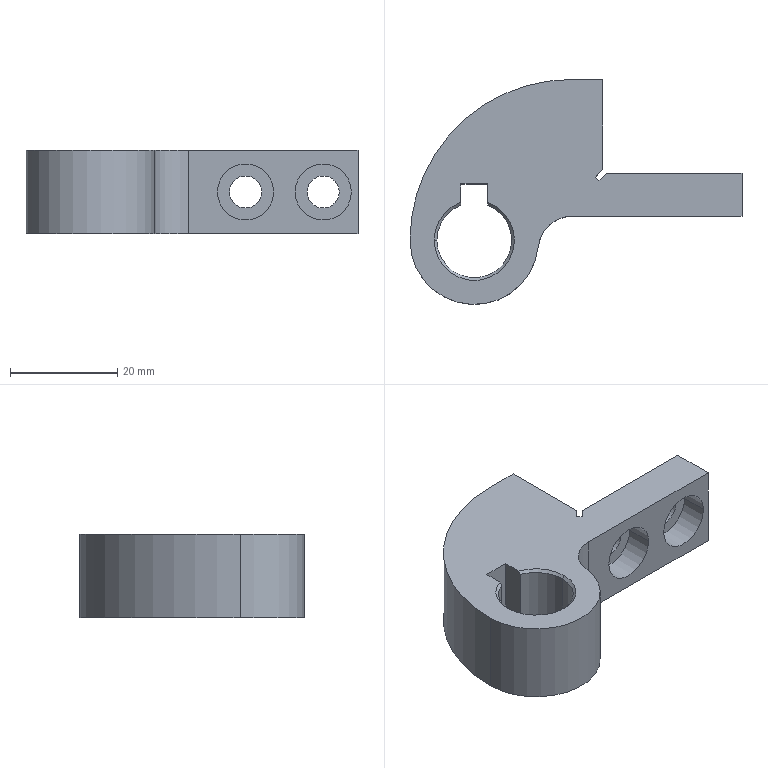Part | SolidWorks | features ICE 3, Chamfer 1, Extrusion 1 | 1 solid | 35 faces | box 62 x 42 x 15.5 mm | volume 16029 mm3 | plane 15 | cylinder 14 | cone 6 | commonest cylinder face diameters 6 x4 10.5 x4 14 x3 13 x1 24 x1 60 x1
STEP:
#1=CARTESIAN_POINT('',(-7.,0.,7.25));
#2=VERTEX_POINT('',#1);
#3=CARTESIAN_POINT('',(7.,0.,7.25));
#4=VERTEX_POINT('',#3);
#5=CARTESIAN_POINT('',(0.,0.,7.25));
#6=DIRECTION('',(0.,0.,1.));
#7=DIRECTION('',(1.,0.,0.));
#8=AXIS2_PLACEMENT_3D('',#5,#6,#7);
#9=CIRCLE('',#8,7.);
#10=EDGE_CURVE('',#2,#4,#9,.T.);
#11=ORIENTED_EDGE('',*,*,#10,.F.);
#12=CARTESIAN_POINT('',(-7.5,0.,7.75));
#13=VERTEX_POINT('',#12);
#14=CARTESIAN_POINT('',(-7.,0.,7.25));
#15=DIRECTION('',(-0.7071,0.,0.7071));
#16=VECTOR('',#15,1000.);
#17=LINE('',#14,#16);
#18=EDGE_CURVE('',#2,#13,#17,.T.);
#19=ORIENTED_EDGE('',*,*,#18,.T.);
#20=CARTESIAN_POINT('',(7.5,0.,7.75));
#21=VERTEX_POINT('',#20);
#22=CARTESIAN_POINT('',(0.,0.,7.75));
#23=DIRECTION('',(0.,0.,-1.));
#24=DIRECTION('',(1.,0.,0.));
#25=AXIS2_PLACEMENT_3D('',#22,#23,#24);
#26=CIRCLE('',#25,7.5);
#27=EDGE_CURVE('',#21,#13,#26,.T.);
#28=ORIENTED_EDGE('',*,*,#27,.F.);
#29=CARTESIAN_POINT('',(7.,0.,7.25));
#30=DIRECTION('',(0.7071,0.,0.7071));
#31=VECTOR('',#30,1000.);
#32=LINE('',#29,#31);
#33=EDGE_CURVE('',#4,#21,#32,.T.);
#34=ORIENTED_EDGE('',*,*,#33,.F.);
#35=EDGE_LOOP('',(#11,#19,#28,#34));
#36=FACE_OUTER_BOUND('',#35,.T.);
#37=CARTESIAN_POINT('',(0.,0.,7.25));
#38=DIRECTION('',(0.,0.,1.));
#39=DIRECTION('',(1.,0.,0.));
#40=AXIS2_PLACEMENT_3D('',#37,#38,#39);
#41=CONICAL_SURFACE('',#40,7.,0.7854);
#42=ADVANCED_FACE('',(#36),#41,.F.);
#43=CARTESIAN_POINT('',(2.5,6.538,7.25));
#44=VERTEX_POINT('',#43);
#45=CARTESIAN_POINT('',(0.,0.,7.25));
#46=DIRECTION('',(0.,0.,1.));
#47=DIRECTION('',(1.,0.,0.));
#48=AXIS2_PLACEMENT_3D('',#45,#46,#47);
#49=CIRCLE('',#48,7.);
#50=EDGE_CURVE('',#4,#44,#49,.T.);
#51=ORIENTED_EDGE('',*,*,#50,.F.);
#52=ORIENTED_EDGE('',*,*,#33,.T.);
#53=CARTESIAN_POINT('',(2.5,7.071,7.75));
#54=VERTEX_POINT('',#53);
#55=CARTESIAN_POINT('',(0.,0.,7.75));
#56=DIRECTION('',(0.,0.,-1.));
#57=DIRECTION('',(1.,0.,0.));
#58=AXIS2_PLACEMENT_3D('',#55,#56,#57);
#59=CIRCLE('',#58,7.5);
#60=EDGE_CURVE('',#54,#21,#59,.T.);
#61=ORIENTED_EDGE('',*,*,#60,.F.);
#62=CARTESIAN_POINT('',(2.5,6.538,7.25));
#63=CARTESIAN_POINT('',(2.5,6.716,7.416));
#64=CARTESIAN_POINT('',(2.5,6.894,7.583));
#65=CARTESIAN_POINT('',(2.5,7.071,7.75));
#66=B_SPLINE_CURVE_WITH_KNOTS('',3,(#62,#63,#64,#65),.UNSPECIFIED.,.F.,.F.,(4,4),(0.,0.0007306),.UNSPECIFIED.);
#67=EDGE_CURVE('',#44,#54,#66,.T.);
#68=ORIENTED_EDGE('',*,*,#67,.F.);
#69=EDGE_LOOP('',(#51,#52,#61,#68));
#70=FACE_OUTER_BOUND('',#69,.T.);
#71=CARTESIAN_POINT('',(0.,0.,7.25));
#72=DIRECTION('',(0.,0.,1.));
#73=DIRECTION('',(1.,0.,0.));
#74=AXIS2_PLACEMENT_3D('',#71,#72,#73);
#75=CONICAL_SURFACE('',#74,7.,0.7854);
#76=ADVANCED_FACE('',(#70),#75,.F.);
#77=CARTESIAN_POINT('',(7.,0.,-7.25));
#78=VERTEX_POINT('',#77);
#79=CARTESIAN_POINT('',(-7.,0.,-7.25));
#80=VERTEX_POINT('',#79);
#81=CARTESIAN_POINT('',(0.,0.,-7.25));
#82=DIRECTION('',(0.,0.,-1.));
#83=DIRECTION('',(1.,0.,0.));
#84=AXIS2_PLACEMENT_3D('',#81,#82,#83);
#85=CIRCLE('',#84,7.);
#86=EDGE_CURVE('',#78,#80,#85,.T.);
#87=ORIENTED_EDGE('',*,*,#86,.F.);
#88=CARTESIAN_POINT('',(7.5,0.,-7.75));
#89=VERTEX_POINT('',#88);
#90=CARTESIAN_POINT('',(7.5,0.,-7.75));
#91=DIRECTION('',(0.7071,0.,-0.7071));
#92=VECTOR('',#91,1000.);
#93=LINE('',#90,#92);
#94=EDGE_CURVE('',#78,#89,#93,.T.);
#95=ORIENTED_EDGE('',*,*,#94,.T.);
#96=CARTESIAN_POINT('',(-7.5,0.,-7.75));
#97=VERTEX_POINT('',#96);
#98=CARTESIAN_POINT('',(0.,0.,-7.75));
#99=DIRECTION('',(0.,0.,1.));
#100=DIRECTION('',(1.,0.,0.));
#101=AXIS2_PLACEMENT_3D('',#98,#99,#100);
#102=CIRCLE('',#101,7.5);
#103=EDGE_CURVE('',#97,#89,#102,.T.);
#104=ORIENTED_EDGE('',*,*,#103,.F.);
#105=CARTESIAN_POINT('',(-7.5,0.,-7.75));
#106=DIRECTION('',(-0.7071,0.,-0.7071));
#107=VECTOR('',#106,1000.);
#108=LINE('',#105,#107);
#109=EDGE_CURVE('',#80,#97,#108,.T.);
#110=ORIENTED_EDGE('',*,*,#109,.F.);
#111=EDGE_LOOP('',(#87,#95,#104,#110));
#112=FACE_OUTER_BOUND('',#111,.T.);
#113=CARTESIAN_POINT('',(0.,0.,-7.75));
#114=DIRECTION('',(0.,0.,-1.));
#115=DIRECTION('',(-1.,0.,0.));
#116=AXIS2_PLACEMENT_3D('',#113,#114,#115);
#117=CONICAL_SURFACE('',#116,7.5,0.7854);
#118=ADVANCED_FACE('',(#112),#117,.F.);
#119=CARTESIAN_POINT('',(-2.5,6.538,-7.25));
#120=VERTEX_POINT('',#119);
#121=CARTESIAN_POINT('',(0.,0.,-7.25));
#122=DIRECTION('',(0.,0.,-1.));
#123=DIRECTION('',(1.,0.,0.));
#124=AXIS2_PLACEMENT_3D('',#121,#122,#123);
#125=CIRCLE('',#124,7.);
#126=EDGE_CURVE('',#80,#120,#125,.T.);
#127=ORIENTED_EDGE('',*,*,#126,.F.);
#128=ORIENTED_EDGE('',*,*,#109,.T.);
#129=CARTESIAN_POINT('',(-2.5,7.071,-7.75));
#130=VERTEX_POINT('',#129);
#131=CARTESIAN_POINT('',(0.,0.,-7.75));
#132=DIRECTION('',(0.,0.,1.));
#133=DIRECTION('',(1.,0.,0.));
#134=AXIS2_PLACEMENT_3D('',#131,#132,#133);
#135=CIRCLE('',#134,7.5);
#136=EDGE_CURVE('',#130,#97,#135,.T.);
#137=ORIENTED_EDGE('',*,*,#136,.F.);
#138=CARTESIAN_POINT('',(-2.5,6.538,-7.25));
#139=CARTESIAN_POINT('',(-2.5,6.716,-7.416));
#140=CARTESIAN_POINT('',(-2.5,6.894,-7.583));
#141=CARTESIAN_POINT('',(-2.5,7.071,-7.75));
#142=B_SPLINE_CURVE_WITH_KNOTS('',3,(#138,#139,#140,#141),.UNSPECIFIED.,.F.,.F.,(4,4),(0.,0.0007306),.UNSPECIFIED.);
#143=EDGE_CURVE('',#120,#130,#142,.T.);
#144=ORIENTED_EDGE('',*,*,#143,.F.);
#145=EDGE_LOOP('',(#127,#128,#137,#144));
#146=FACE_OUTER_BOUND('',#145,.T.);
#147=CARTESIAN_POINT('',(0.,0.,-7.75));
#148=DIRECTION('',(0.,0.,-1.));
#149=DIRECTION('',(-1.,0.,0.));
#150=AXIS2_PLACEMENT_3D('',#147,#148,#149);
#151=CONICAL_SURFACE('',#150,7.5,0.7854);
#152=ADVANCED_FACE('',(#146),#151,.F.);
#153=CARTESIAN_POINT('',(38.25,9.5,0.));
#154=VERTEX_POINT('',#153);
#155=CARTESIAN_POINT('',(48.75,9.5,0.));
#156=VERTEX_POINT('',#155);
#157=CARTESIAN_POINT('',(43.5,9.5,0.));
#158=DIRECTION('',(0.,-1.,0.));
#159=DIRECTION('',(1.,0.,0.));
#160=AXIS2_PLACEMENT_3D('',#157,#158,#159);
#161=CIRCLE('',#160,5.25);
#162=EDGE_CURVE('',#154,#156,#161,.T.);
#163=ORIENTED_EDGE('',*,*,#162,.F.);
#164=CARTESIAN_POINT('',(38.25,4.5,0.));
#165=VERTEX_POINT('',#164);
#166=CARTESIAN_POINT('',(38.25,9.5,0.));
#167=DIRECTION('',(0.,-1.,0.));
#168=VECTOR('',#167,1000.);
#169=LINE('',#166,#168);
#170=EDGE_CURVE('',#154,#165,#169,.T.);
#171=ORIENTED_EDGE('',*,*,#170,.T.);
#172=CARTESIAN_POINT('',(48.75,4.5,0.));
#173=VERTEX_POINT('',#172);
#174=CARTESIAN_POINT('',(43.5,4.5,0.));
#175=DIRECTION('',(0.,-1.,0.));
#176=DIRECTION('',(1.,0.,0.));
#177=AXIS2_PLACEMENT_3D('',#174,#175,#176);
#178=CIRCLE('',#177,5.25);
#179=EDGE_CURVE('',#165,#173,#178,.T.);
#180=ORIENTED_EDGE('',*,*,#179,.T.);
#181=CARTESIAN_POINT('',(48.75,9.5,0.));
#182=DIRECTION('',(0.,-1.,0.));
#183=VECTOR('',#182,1000.);
#184=LINE('',#181,#183);
#185=EDGE_CURVE('',#156,#173,#184,.T.);
#186=ORIENTED_EDGE('',*,*,#185,.F.);
#187=EDGE_LOOP('',(#163,#171,#180,#186));
#188=FACE_OUTER_BOUND('',#187,.T.);
#189=CARTESIAN_POINT('',(43.5,9.5,0.));
#190=DIRECTION('',(0.,-1.,0.));
#191=DIRECTION('',(1.,0.,0.));
#192=AXIS2_PLACEMENT_3D('',#189,#190,#191);
#193=CYLINDRICAL_SURFACE('',#192,5.25);
#194=ADVANCED_FACE('',(#188),#193,.F.);
#195=CARTESIAN_POINT('',(23.75,9.5,0.));
#196=VERTEX_POINT('',#195);
#197=CARTESIAN_POINT('',(34.25,9.5,0.));
#198=VERTEX_POINT('',#197);
#199=CARTESIAN_POINT('',(29.,9.5,0.));
#200=DIRECTION('',(0.,-1.,0.));
#201=DIRECTION('',(1.,0.,0.));
#202=AXIS2_PLACEMENT_3D('',#199,#200,#201);
#203=CIRCLE('',#202,5.25);
#204=EDGE_CURVE('',#196,#198,#203,.T.);
#205=ORIENTED_EDGE('',*,*,#204,.F.);
#206=CARTESIAN_POINT('',(23.75,4.5,0.));
#207=VERTEX_POINT('',#206);
#208=CARTESIAN_POINT('',(23.75,9.5,0.));
#209=DIRECTION('',(0.,-1.,0.));
#210=VECTOR('',#209,1000.);
#211=LINE('',#208,#210);
#212=EDGE_CURVE('',#196,#207,#211,.T.);
#213=ORIENTED_EDGE('',*,*,#212,.T.);
#214=CARTESIAN_POINT('',(34.25,4.5,0.));
#215=VERTEX_POINT('',#214);
#216=CARTESIAN_POINT('',(29.,4.5,0.));
#217=DIRECTION('',(0.,-1.,0.));
#218=DIRECTION('',(1.,0.,0.));
#219=AXIS2_PLACEMENT_3D('',#216,#217,#218);
#220=CIRCLE('',#219,5.25);
#221=EDGE_CURVE('',#207,#215,#220,.T.);
#222=ORIENTED_EDGE('',*,*,#221,.T.);
#223=CARTESIAN_POINT('',(34.25,9.5,0.));
#224=DIRECTION('',(0.,-1.,0.));
#225=VECTOR('',#224,1000.);
#226=LINE('',#223,#225);
#227=EDGE_CURVE('',#198,#215,#226,.T.);
#228=ORIENTED_EDGE('',*,*,#227,.F.);
#229=EDGE_LOOP('',(#205,#213,#222,#228));
#230=FACE_OUTER_BOUND('',#229,.T.);
#231=CARTESIAN_POINT('',(29.,9.5,0.));
#232=DIRECTION('',(0.,-1.,0.));
#233=DIRECTION('',(1.,0.,0.));
#234=AXIS2_PLACEMENT_3D('',#231,#232,#233);
#235=CYLINDRICAL_SURFACE('',#234,5.25);
#236=ADVANCED_FACE('',(#230),#235,.F.);
#237=ORIENTED_EDGE('',*,*,#10,.T.);
#238=CARTESIAN_POINT('',(7.,0.,7.75));
#239=DIRECTION('',(0.,0.,-1.));
#240=VECTOR('',#239,1000.);
#241=LINE('',#238,#240);
#242=EDGE_CURVE('',#4,#78,#241,.T.);
#243=ORIENTED_EDGE('',*,*,#242,.T.);
#244=ORIENTED_EDGE('',*,*,#86,.T.);
#245=CARTESIAN_POINT('',(-7.,0.,7.75));
#246=DIRECTION('',(0.,0.,-1.));
#247=VECTOR('',#246,1000.);
#248=LINE('',#245,#247);
#249=EDGE_CURVE('',#2,#80,#248,.T.);
#250=ORIENTED_EDGE('',*,*,#249,.F.);
#251=EDGE_LOOP('',(#237,#243,#244,#250));
#252=FACE_OUTER_BOUND('',#251,.T.);
#253=CARTESIAN_POINT('',(0.,0.,7.75));
#254=DIRECTION('',(0.,0.,-1.));
#255=DIRECTION('',(-1.,0.,0.));
#256=AXIS2_PLACEMENT_3D('',#253,#254,#255);
#257=CYLINDRICAL_SURFACE('',#256,7.);
#258=ADVANCED_FACE('',(#252),#257,.F.);
#259=CARTESIAN_POINT('',(-2.5,6.538,7.25));
#260=VERTEX_POINT('',#259);
#261=CARTESIAN_POINT('',(0.,0.,7.25));
#262=DIRECTION('',(0.,0.,1.));
#263=DIRECTION('',(1.,0.,0.));
#264=AXIS2_PLACEMENT_3D('',#261,#262,#263);
#265=CIRCLE('',#264,7.);
#266=EDGE_CURVE('',#260,#2,#265,.T.);
#267=ORIENTED_EDGE('',*,*,#266,.T.);
#268=ORIENTED_EDGE('',*,*,#249,.T.);
#269=ORIENTED_EDGE('',*,*,#126,.T.);
#270=CARTESIAN_POINT('',(-2.5,6.538,7.75));
#271=DIRECTION('',(0.,0.,-1.));
#272=VECTOR('',#271,1000.);
#273=LINE('',#270,#272);
#274=EDGE_CURVE('',#260,#120,#273,.T.);
#275=ORIENTED_EDGE('',*,*,#274,.F.);
#276=EDGE_LOOP('',(#267,#268,#269,#275));
#277=FACE_OUTER_BOUND('',#276,.T.);
#278=CARTESIAN_POINT('',(0.,0.,7.75));
#279=DIRECTION('',(0.,0.,-1.));
#280=DIRECTION('',(-1.,0.,0.));
#281=AXIS2_PLACEMENT_3D('',#278,#279,#280);
#282=CYLINDRICAL_SURFACE('',#281,7.);
#283=ADVANCED_FACE('',(#277),#282,.F.);
#284=CARTESIAN_POINT('',(32.,9.5,0.));
#285=VERTEX_POINT('',#284);
#286=CARTESIAN_POINT('',(26.,9.5,0.));
#287=VERTEX_POINT('',#286);
#288=CARTESIAN_POINT('',(29.,9.5,0.));
#289=DIRECTION('',(0.,1.,0.));
#290=DIRECTION('',(1.,0.,0.));
#291=AXIS2_PLACEMENT_3D('',#288,#289,#290);
#292=CIRCLE('',#291,3.);
#293=EDGE_CURVE('',#285,#287,#292,.T.);
#294=ORIENTED_EDGE('',*,*,#293,.F.);
#295=CARTESIAN_POINT('',(32.,12.5,0.));
#296=VERTEX_POINT('',#295);
#297=CARTESIAN_POINT('',(32.,-12.,0.));
#298=DIRECTION('',(0.,1.,0.));
#299=VECTOR('',#298,1000.);
#300=LINE('',#297,#299);
#301=EDGE_CURVE('',#285,#296,#300,.T.);
#302=ORIENTED_EDGE('',*,*,#301,.T.);
#303=CARTESIAN_POINT('',(26.,12.5,0.));
#304=VERTEX_POINT('',#303);
#305=CARTESIAN_POINT('',(29.,12.5,0.));
#306=DIRECTION('',(0.,-1.,0.));
#307=DIRECTION('',(1.,0.,0.));
#308=AXIS2_PLACEMENT_3D('',#305,#306,#307);
#309=CIRCLE('',#308,3.);
#310=EDGE_CURVE('',#304,#296,#309,.T.);
#311=ORIENTED_EDGE('',*,*,#310,.F.);
#312=CARTESIAN_POINT('',(26.,-12.,0.));
#313=DIRECTION('',(0.,1.,0.));
#314=VECTOR('',#313,1000.);
#315=LINE('',#312,#314);
#316=EDGE_CURVE('',#287,#304,#315,.T.);
#317=ORIENTED_EDGE('',*,*,#316,.F.);
#318=EDGE_LOOP('',(#294,#302,#311,#317));
#319=FACE_OUTER_BOUND('',#318,.T.);
#320=CARTESIAN_POINT('',(29.,-12.,0.));
#321=DIRECTION('',(0.,1.,0.));
#322=DIRECTION('',(-1.,0.,0.));
#323=AXIS2_PLACEMENT_3D('',#320,#321,#322);
#324=CYLINDRICAL_SURFACE('',#323,3.);
#325=ADVANCED_FACE('',(#319),#324,.F.);
#326=CARTESIAN_POINT('',(46.5,9.5,0.));
#327=VERTEX_POINT('',#326);
#328=CARTESIAN_POINT('',(40.5,9.5,0.));
#329=VERTEX_POINT('',#328);
#330=CARTESIAN_POINT('',(43.5,9.5,0.));
#331=DIRECTION('',(0.,1.,0.));
#332=DIRECTION('',(1.,0.,0.));
#333=AXIS2_PLACEMENT_3D('',#330,#331,#332);
#334=CIRCLE('',#333,3.);
#335=EDGE_CURVE('',#327,#329,#334,.T.);
#336=ORIENTED_EDGE('',*,*,#335,.F.);
#337=CARTESIAN_POINT('',(46.5,12.5,0.));
#338=VERTEX_POINT('',#337);
#339=CARTESIAN_POINT('',(46.5,-12.,0.));
#340=DIRECTION('',(0.,1.,0.));
#341=VECTOR('',#340,1000.);
#342=LINE('',#339,#341);
#343=EDGE_CURVE('',#327,#338,#342,.T.);
#344=ORIENTED_EDGE('',*,*,#343,.T.);
#345=CARTESIAN_POINT('',(40.5,12.5,0.));
#346=VERTEX_POINT('',#345);
#347=CARTESIAN_POINT('',(43.5,12.5,0.));
#348=DIRECTION('',(0.,-1.,0.));
#349=DIRECTION('',(1.,0.,0.));
#350=AXIS2_PLACEMENT_3D('',#347,#348,#349);
#351=CIRCLE('',#350,3.);
#352=EDGE_CURVE('',#346,#338,#351,.T.);
#353=ORIENTED_EDGE('',*,*,#352,.F.);
#354=CARTESIAN_POINT('',(40.5,-12.,0.));
#355=DIRECTION('',(0.,1.,0.));
#356=VECTOR('',#355,1000.);
#357=LINE('',#354,#356);
#358=EDGE_CURVE('',#329,#346,#357,.T.);
#359=ORIENTED_EDGE('',*,*,#358,.F.);
#360=EDGE_LOOP('',(#336,#344,#353,#359));
#361=FACE_OUTER_BOUND('',#360,.T.);
#362=CARTESIAN_POINT('',(43.5,-12.,0.));
#363=DIRECTION('',(0.,1.,0.));
#364=DIRECTION('',(-1.,0.,0.));
#365=AXIS2_PLACEMENT_3D('',#362,#363,#364);
#366=CYLINDRICAL_SURFACE('',#365,3.);
#367=ADVANCED_FACE('',(#361),#366,.F.);
#368=ORIENTED_EDGE('',*,*,#343,.F.);
#369=CARTESIAN_POINT('',(43.5,9.5,0.));
#370=DIRECTION('',(0.,1.,0.));
#371=DIRECTION('',(1.,0.,0.));
#372=AXIS2_PLACEMENT_3D('',#369,#370,#371);
#373=CIRCLE('',#372,3.);
#374=EDGE_CURVE('',#329,#327,#373,.T.);
#375=ORIENTED_EDGE('',*,*,#374,.F.);
#376=ORIENTED_EDGE('',*,*,#358,.T.);
#377=CARTESIAN_POINT('',(43.5,12.5,0.));
#378=DIRECTION('',(0.,-1.,0.));
#379=DIRECTION('',(1.,0.,0.));
#380=AXIS2_PLACEMENT_3D('',#377,#378,#379);
#381=CIRCLE('',#380,3.);
#382=EDGE_CURVE('',#338,#346,#381,.T.);
#383=ORIENTED_EDGE('',*,*,#382,.F.);
#384=EDGE_LOOP('',(#368,#375,#376,#383));
#385=FACE_OUTER_BOUND('',#384,.T.);
#386=CARTESIAN_POINT('',(43.5,-12.,0.));
#387=DIRECTION('',(0.,1.,0.));
#388=DIRECTION('',(-1.,0.,0.));
#389=AXIS2_PLACEMENT_3D('',#386,#387,#388);
#390=CYLINDRICAL_SURFACE('',#389,3.);
#391=ADVANCED_FACE('',(#385),#390,.F.);
#392=ORIENTED_EDGE('',*,*,#301,.F.);
#393=CARTESIAN_POINT('',(29.,9.5,0.));
#394=DIRECTION('',(0.,1.,0.));
#395=DIRECTION('',(1.,0.,0.));
#396=AXIS2_PLACEMENT_3D('',#393,#394,#395);
#397=CIRCLE('',#396,3.);
#398=EDGE_CURVE('',#287,#285,#397,.T.);
#399=ORIENTED_EDGE('',*,*,#398,.F.);
#400=ORIENTED_EDGE('',*,*,#316,.T.);
#401=CARTESIAN_POINT('',(29.,12.5,0.));
#402=DIRECTION('',(0.,-1.,0.));
#403=DIRECTION('',(1.,0.,0.));
#404=AXIS2_PLACEMENT_3D('',#401,#402,#403);
#405=CIRCLE('',#404,3.);
#406=EDGE_CURVE('',#296,#304,#405,.T.);
#407=ORIENTED_EDGE('',*,*,#406,.F.);
#408=EDGE_LOOP('',(#392,#399,#400,#407));
#409=FACE_OUTER_BOUND('',#408,.T.);
#410=CARTESIAN_POINT('',(29.,-12.,0.));
#411=DIRECTION('',(0.,1.,0.));
#412=DIRECTION('',(-1.,0.,0.));
#413=AXIS2_PLACEMENT_3D('',#410,#411,#412);
#414=CYLINDRICAL_SURFACE('',#413,3.);
#415=ADVANCED_FACE('',(#409),#414,.F.);
#416=CARTESIAN_POINT('',(23.293,11.086,7.75));
#417=VERTEX_POINT('',#416);
#418=CARTESIAN_POINT('',(24.707,12.5,7.75));
#419=VERTEX_POINT('',#418);
#420=CARTESIAN_POINT('',(14.299,2.092,7.75));
#421=DIRECTION('',(0.7071,0.7071,0.));
#422=VECTOR('',#421,1000.);
#423=LINE('',#420,#422);
#424=EDGE_CURVE('',#417,#419,#423,.T.);
#425=ORIENTED_EDGE('',*,*,#424,.F.);
#426=CARTESIAN_POINT('',(22.586,11.793,7.75));
#427=VERTEX_POINT('',#426);
#428=CARTESIAN_POINT('',(27.385,6.994,7.75));
#429=DIRECTION('',(0.7071,-0.7071,0.));
#430=VECTOR('',#429,1000.);
#431=LINE('',#428,#430);
#432=EDGE_CURVE('',#427,#417,#431,.T.);
#433=ORIENTED_EDGE('',*,*,#432,.F.);
#434=CARTESIAN_POINT('',(24.,13.207,7.75));
#435=VERTEX_POINT('',#434);
#436=CARTESIAN_POINT('',(13.592,2.799,7.75));
#437=DIRECTION('',(-0.7071,-0.7071,0.));
#438=VECTOR('',#437,1000.);
#439=LINE('',#436,#438);
#440=EDGE_CURVE('',#435,#427,#439,.T.);
#441=ORIENTED_EDGE('',*,*,#440,.F.);
#442=CARTESIAN_POINT('',(24.,30.,7.75));
#443=VERTEX_POINT('',#442);
#444=CARTESIAN_POINT('',(24.,30.,7.75));
#445=DIRECTION('',(0.,1.,0.));
#446=VECTOR('',#445,1000.);
#447=LINE('',#444,#446);
#448=EDGE_CURVE('',#435,#443,#447,.T.);
#449=ORIENTED_EDGE('',*,*,#448,.T.);
#450=CARTESIAN_POINT('',(18.,30.,7.75));
#451=VERTEX_POINT('',#450);
#452=CARTESIAN_POINT('',(18.,30.,7.75));
#453=DIRECTION('',(-1.,0.,0.));
#454=VECTOR('',#453,1000.);
#455=LINE('',#452,#454);
#456=EDGE_CURVE('',#443,#451,#455,.T.);
#457=ORIENTED_EDGE('',*,*,#456,.T.);
#458=CARTESIAN_POINT('',(-12.,0.,7.75));
#459=VERTEX_POINT('',#458);
#460=CARTESIAN_POINT('',(18.,0.,7.75));
#461=DIRECTION('',(0.,0.,1.));
#462=DIRECTION('',(-1.,0.,0.));
#463=AXIS2_PLACEMENT_3D('',#460,#461,#462);
#464=CIRCLE('',#463,30.);
#465=EDGE_CURVE('',#451,#459,#464,.T.);
#466=ORIENTED_EDGE('',*,*,#465,.T.);
#467=CARTESIAN_POINT('',(11.93,-1.297,7.75));
#468=VERTEX_POINT('',#467);
#469=CARTESIAN_POINT('',(0.,0.,7.75));
#470=DIRECTION('',(0.,0.,1.));
#471=DIRECTION('',(-1.,0.,0.));
#472=AXIS2_PLACEMENT_3D('',#469,#470,#471);
#473=CIRCLE('',#472,12.);
#474=EDGE_CURVE('',#459,#468,#473,.T.);
#475=ORIENTED_EDGE('',*,*,#474,.T.);
#476=CARTESIAN_POINT('',(18.392,4.5,7.75));
#477=VERTEX_POINT('',#476);
#478=CARTESIAN_POINT('',(18.392,-2.,7.75));
#479=DIRECTION('',(0.,0.,-1.));
#480=DIRECTION('',(1.,0.,0.));
#481=AXIS2_PLACEMENT_3D('',#478,#479,#480);
#482=CIRCLE('',#481,6.5);
#483=EDGE_CURVE('',#468,#477,#482,.T.);
#484=ORIENTED_EDGE('',*,*,#483,.T.);
#485=CARTESIAN_POINT('',(50.,4.5,7.75));
#486=VERTEX_POINT('',#485);
#487=CARTESIAN_POINT('',(50.,4.5,7.75));
#488=DIRECTION('',(1.,0.,0.));
#489=VECTOR('',#488,1000.);
#490=LINE('',#487,#489);
#491=EDGE_CURVE('',#477,#486,#490,.T.);
#492=ORIENTED_EDGE('',*,*,#491,.T.);
#493=CARTESIAN_POINT('',(50.,12.5,7.75));
#494=VERTEX_POINT('',#493);
#495=CARTESIAN_POINT('',(50.,12.5,7.75));
#496=DIRECTION('',(0.,1.,0.));
#497=VECTOR('',#496,1000.);
#498=LINE('',#495,#497);
#499=EDGE_CURVE('',#486,#494,#498,.T.);
#500=ORIENTED_EDGE('',*,*,#499,.T.);
#501=CARTESIAN_POINT('',(24.,12.5,7.75));
#502=DIRECTION('',(-1.,0.,0.));
#503=VECTOR('',#502,1000.);
#504=LINE('',#501,#503);
#505=EDGE_CURVE('',#494,#419,#504,.T.);
#506=ORIENTED_EDGE('',*,*,#505,.T.);
#507=EDGE_LOOP('',(#425,#433,#441,#449,#457,#466,#475,#484,#492,#500,#506));
#508=FACE_OUTER_BOUND('',#507,.T.);
#509=CARTESIAN_POINT('',(2.5,10.5,7.75));
#510=VERTEX_POINT('',#509);
#511=CARTESIAN_POINT('',(2.5,6.538,7.75));
#512=DIRECTION('',(0.,1.,0.));
#513=VECTOR('',#512,1000.);
#514=LINE('',#511,#513);
#515=EDGE_CURVE('',#54,#510,#514,.T.);
#516=ORIENTED_EDGE('',*,*,#515,.F.);
#517=ORIENTED_EDGE('',*,*,#60,.T.);
#518=ORIENTED_EDGE('',*,*,#27,.T.);
#519=CARTESIAN_POINT('',(-2.5,7.071,7.75));
#520=VERTEX_POINT('',#519);
#521=CARTESIAN_POINT('',(0.,0.,7.75));
#522=DIRECTION('',(0.,0.,-1.));
#523=DIRECTION('',(1.,0.,0.));
#524=AXIS2_PLACEMENT_3D('',#521,#522,#523);
#525=CIRCLE('',#524,7.5);
#526=EDGE_CURVE('',#13,#520,#525,.T.);
#527=ORIENTED_EDGE('',*,*,#526,.T.);
#528=CARTESIAN_POINT('',(-2.5,10.5,7.75));
#529=VERTEX_POINT('',#528);
#530=CARTESIAN_POINT('',(-2.5,6.538,7.75));
#531=DIRECTION('',(0.,-1.,0.));
#532=VECTOR('',#531,1000.);
#533=LINE('',#530,#532);
#534=EDGE_CURVE('',#529,#520,#533,.T.);
#535=ORIENTED_EDGE('',*,*,#534,.F.);
#536=CARTESIAN_POINT('',(-2.5,10.5,7.75));
#537=DIRECTION('',(-1.,0.,0.));
#538=VECTOR('',#537,1000.);
#539=LINE('',#536,#538);
#540=EDGE_CURVE('',#510,#529,#539,.T.);
#541=ORIENTED_EDGE('',*,*,#540,.F.);
#542=EDGE_LOOP('',(#516,#517,#518,#527,#535,#541));
#543=FACE_BOUND('',#542,.T.);
#544=CARTESIAN_POINT('',(18.392,-2.,7.75));
#545=DIRECTION('',(0.,0.,1.));
#546=DIRECTION('',(1.,0.,0.));
#547=AXIS2_PLACEMENT_3D('',#544,#545,#546);
#548=PLANE('',#547);
#549=ADVANCED_FACE('',(#508,#543),#548,.T.);
#550=CARTESIAN_POINT('',(22.586,11.793,-7.75));
#551=VERTEX_POINT('',#550);
#552=CARTESIAN_POINT('',(23.293,11.086,-7.75));
#553=VERTEX_POINT('',#552);
#554=CARTESIAN_POINT('',(22.586,11.793,-7.75));
#555=DIRECTION('',(0.7071,-0.7071,0.));
#556=VECTOR('',#555,1000.);
#557=LINE('',#554,#556);
#558=EDGE_CURVE('',#551,#553,#557,.T.);
#559=ORIENTED_EDGE('',*,*,#558,.T.);
#560=CARTESIAN_POINT('',(24.707,12.5,-7.75));
#561=VERTEX_POINT('',#560);
#562=CARTESIAN_POINT('',(24.707,12.5,-7.75));
#563=DIRECTION('',(0.7071,0.7071,0.));
#564=VECTOR('',#563,1000.);
#565=LINE('',#562,#564);
#566=EDGE_CURVE('',#553,#561,#565,.T.);
#567=ORIENTED_EDGE('',*,*,#566,.T.);
#568=CARTESIAN_POINT('',(50.,12.5,-7.75));
#569=VERTEX_POINT('',#568);
#570=CARTESIAN_POINT('',(24.,12.5,-7.75));
#571=DIRECTION('',(-1.,0.,0.));
#572=VECTOR('',#571,1000.);
#573=LINE('',#570,#572);
#574=EDGE_CURVE('',#569,#561,#573,.T.);
#575=ORIENTED_EDGE('',*,*,#574,.F.);
#576=CARTESIAN_POINT('',(50.,4.5,-7.75));
#577=VERTEX_POINT('',#576);
#578=CARTESIAN_POINT('',(50.,12.5,-7.75));
#579=DIRECTION('',(0.,1.,0.));
#580=VECTOR('',#579,1000.);
#581=LINE('',#578,#580);
#582=EDGE_CURVE('',#577,#569,#581,.T.);
#583=ORIENTED_EDGE('',*,*,#582,.F.);
#584=CARTESIAN_POINT('',(18.392,4.5,-7.75));
#585=VERTEX_POINT('',#584);
#586=CARTESIAN_POINT('',(50.,4.5,-7.75));
#587=DIRECTION('',(1.,0.,0.));
#588=VECTOR('',#587,1000.);
#589=LINE('',#586,#588);
#590=EDGE_CURVE('',#585,#577,#589,.T.);
#591=ORIENTED_EDGE('',*,*,#590,.F.);
#592=CARTESIAN_POINT('',(11.93,-1.297,-7.75));
#593=VERTEX_POINT('',#592);
#594=CARTESIAN_POINT('',(18.392,-2.,-7.75));
#595=DIRECTION('',(0.,0.,-1.));
#596=DIRECTION('',(1.,0.,0.));
#597=AXIS2_PLACEMENT_3D('',#594,#595,#596);
#598=CIRCLE('',#597,6.5);
#599=EDGE_CURVE('',#593,#585,#598,.T.);
#600=ORIENTED_EDGE('',*,*,#599,.F.);
#601=CARTESIAN_POINT('',(-12.,0.,-7.75));
#602=VERTEX_POINT('',#601);
#603=CARTESIAN_POINT('',(0.,0.,-7.75));
#604=DIRECTION('',(0.,0.,1.));
#605=DIRECTION('',(-1.,0.,0.));
#606=AXIS2_PLACEMENT_3D('',#603,#604,#605);
#607=CIRCLE('',#606,12.);
#608=EDGE_CURVE('',#602,#593,#607,.T.);
#609=ORIENTED_EDGE('',*,*,#608,.F.);
#610=CARTESIAN_POINT('',(18.,30.,-7.75));
#611=VERTEX_POINT('',#610);
#612=CARTESIAN_POINT('',(18.,0.,-7.75));
#613=DIRECTION('',(0.,0.,1.));
#614=DIRECTION('',(-1.,0.,0.));
#615=AXIS2_PLACEMENT_3D('',#612,#613,#614);
#616=CIRCLE('',#615,30.);
#617=EDGE_CURVE('',#611,#602,#616,.T.);
#618=ORIENTED_EDGE('',*,*,#617,.F.);
#619=CARTESIAN_POINT('',(24.,30.,-7.75));
#620=VERTEX_POINT('',#619);
#621=CARTESIAN_POINT('',(18.,30.,-7.75));
#622=DIRECTION('',(-1.,0.,0.));
#623=VECTOR('',#622,1000.);
#624=LINE('',#621,#623);
#625=EDGE_CURVE('',#620,#611,#624,.T.);
#626=ORIENTED_EDGE('',*,*,#625,.F.);
#627=CARTESIAN_POINT('',(24.,13.207,-7.75));
#628=VERTEX_POINT('',#627);
#629=CARTESIAN_POINT('',(24.,30.,-7.75));
#630=DIRECTION('',(0.,1.,0.));
#631=VECTOR('',#630,1000.);
#632=LINE('',#629,#631);
#633=EDGE_CURVE('',#628,#620,#632,.T.);
#634=ORIENTED_EDGE('',*,*,#633,.F.);
#635=CARTESIAN_POINT('',(24.,13.207,-7.75));
#636=DIRECTION('',(-0.7071,-0.7071,0.));
#637=VECTOR('',#636,1000.);
#638=LINE('',#635,#637);
#639=EDGE_CURVE('',#628,#551,#638,.T.);
#640=ORIENTED_EDGE('',*,*,#639,.T.);
#641=EDGE_LOOP('',(#559,#567,#575,#583,#591,#600,#609,#618,#626,#634,#640));
#642=FACE_OUTER_BOUND('',#641,.T.);
#643=CARTESIAN_POINT('',(-2.5,10.5,-7.75));
#644=VERTEX_POINT('',#643);
#645=CARTESIAN_POINT('',(-2.5,6.538,-7.75));
#646=DIRECTION('',(0.,-1.,0.));
#647=VECTOR('',#646,1000.);
#648=LINE('',#645,#647);
#649=EDGE_CURVE('',#644,#130,#648,.T.);
#650=ORIENTED_EDGE('',*,*,#649,.T.);
#651=ORIENTED_EDGE('',*,*,#136,.T.);
#652=ORIENTED_EDGE('',*,*,#103,.T.);
#653=CARTESIAN_POINT('',(2.5,7.071,-7.75));
#654=VERTEX_POINT('',#653);
#655=CARTESIAN_POINT('',(0.,0.,-7.75));
#656=DIRECTION('',(0.,0.,1.));
#657=DIRECTION('',(1.,0.,0.));
#658=AXIS2_PLACEMENT_3D('',#655,#656,#657);
#659=CIRCLE('',#658,7.5);
#660=EDGE_CURVE('',#89,#654,#659,.T.);
#661=ORIENTED_EDGE('',*,*,#660,.T.);
#662=CARTESIAN_POINT('',(2.5,10.5,-7.75));
#663=VERTEX_POINT('',#662);
#664=CARTESIAN_POINT('',(2.5,6.538,-7.75));
#665=DIRECTION('',(0.,1.,0.));
#666=VECTOR('',#665,1000.);
#667=LINE('',#664,#666);
#668=EDGE_CURVE('',#654,#663,#667,.T.);
#669=ORIENTED_EDGE('',*,*,#668,.T.);
#670=CARTESIAN_POINT('',(-2.5,10.5,-7.75));
#671=DIRECTION('',(-1.,0.,0.));
#672=VECTOR('',#671,1000.);
#673=LINE('',#670,#672);
#674=EDGE_CURVE('',#663,#644,#673,.T.);
#675=ORIENTED_EDGE('',*,*,#674,.T.);
#676=EDGE_LOOP('',(#650,#651,#652,#661,#669,#675));
#677=FACE_BOUND('',#676,.T.);
#678=CARTESIAN_POINT('',(18.392,-2.,-7.75));
#679=DIRECTION('',(0.,0.,1.));
#680=DIRECTION('',(1.,0.,0.));
#681=AXIS2_PLACEMENT_3D('',#678,#679,#680);
#682=PLANE('',#681);
#683=ADVANCED_FACE('',(#642,#677),#682,.F.);
#684=ORIENTED_EDGE('',*,*,#599,.T.);
#685=CARTESIAN_POINT('',(18.392,4.5,7.75));
#686=DIRECTION('',(0.,0.,-1.));
#687=VECTOR('',#686,1000.);
#688=LINE('',#685,#687);
#689=EDGE_CURVE('',#477,#585,#688,.T.);
#690=ORIENTED_EDGE('',*,*,#689,.F.);
#691=ORIENTED_EDGE('',*,*,#483,.F.);
#692=CARTESIAN_POINT('',(11.93,-1.297,7.75));
#693=DIRECTION('',(0.,0.,-1.));
#694=VECTOR('',#693,1000.);
#695=LINE('',#692,#694);
#696=EDGE_CURVE('',#468,#593,#695,.T.);
#697=ORIENTED_EDGE('',*,*,#696,.T.);
#698=EDGE_LOOP('',(#684,#690,#691,#697));
#699=FACE_OUTER_BOUND('',#698,.T.);
#700=CARTESIAN_POINT('',(18.392,-2.,7.75));
#701=DIRECTION('',(0.,0.,-1.));
#702=DIRECTION('',(-1.,0.,0.));
#703=AXIS2_PLACEMENT_3D('',#700,#701,#702);
#704=CYLINDRICAL_SURFACE('',#703,6.5);
#705=ADVANCED_FACE('',(#699),#704,.F.);
#706=CARTESIAN_POINT('',(29.,4.5,0.));
#707=DIRECTION('',(0.,-1.,0.));
#708=DIRECTION('',(1.,0.,0.));
#709=AXIS2_PLACEMENT_3D('',#706,#707,#708);
#710=CIRCLE('',#709,5.25);
#711=EDGE_CURVE('',#215,#207,#710,.T.);
#712=ORIENTED_EDGE('',*,*,#711,.F.);
#713=ORIENTED_EDGE('',*,*,#221,.F.);
#714=EDGE_LOOP('',(#712,#713));
#715=FACE_BOUND('',#714,.T.);
#716=CARTESIAN_POINT('',(43.5,4.5,0.));
#717=DIRECTION('',(0.,-1.,0.));
#718=DIRECTION('',(1.,0.,0.));
#719=AXIS2_PLACEMENT_3D('',#716,#717,#718);
#720=CIRCLE('',#719,5.25);
#721=EDGE_CURVE('',#173,#165,#720,.T.);
#722=ORIENTED_EDGE('',*,*,#721,.F.);
#723=ORIENTED_EDGE('',*,*,#179,.F.);
#724=EDGE_LOOP('',(#722,#723));
#725=FACE_BOUND('',#724,.T.);
#726=ORIENTED_EDGE('',*,*,#590,.T.);
#727=CARTESIAN_POINT('',(50.,4.5,7.75));
#728=DIRECTION('',(0.,0.,-1.));
#729=VECTOR('',#728,1000.);
#730=LINE('',#727,#729);
#731=EDGE_CURVE('',#486,#577,#730,.T.);
#732=ORIENTED_EDGE('',*,*,#731,.F.);
#733=ORIENTED_EDGE('',*,*,#491,.F.);
#734=ORIENTED_EDGE('',*,*,#689,.T.);
#735=EDGE_LOOP('',(#726,#732,#733,#734));
#736=FACE_OUTER_BOUND('',#735,.T.);
#737=CARTESIAN_POINT('',(50.,4.5,7.75));
#738=DIRECTION('',(0.,1.,0.));
#739=DIRECTION('',(-1.,0.,0.));
#740=AXIS2_PLACEMENT_3D('',#737,#738,#739);
#741=PLANE('',#740);
#742=ADVANCED_FACE('',(#715,#725,#736),#741,.F.);
#743=ORIENTED_EDGE('',*,*,#582,.T.);
#744=CARTESIAN_POINT('',(50.,12.5,7.75));
#745=DIRECTION('',(0.,0.,-1.));
#746=VECTOR('',#745,1000.);
#747=LINE('',#744,#746);
#748=EDGE_CURVE('',#494,#569,#747,.T.);
#749=ORIENTED_EDGE('',*,*,#748,.F.);
#750=ORIENTED_EDGE('',*,*,#499,.F.);
#751=ORIENTED_EDGE('',*,*,#731,.T.);
#752=EDGE_LOOP('',(#743,#749,#750,#751));
#753=FACE_OUTER_BOUND('',#752,.T.);
#754=CARTESIAN_POINT('',(50.,12.5,7.75));
#755=DIRECTION('',(-1.,0.,0.));
#756=DIRECTION('',(0.,-1.,0.));
#757=AXIS2_PLACEMENT_3D('',#754,#755,#756);
#758=PLANE('',#757);
#759=ADVANCED_FACE('',(#753),#758,.F.);
#760=ORIENTED_EDGE('',*,*,#310,.T.);
#761=ORIENTED_EDGE('',*,*,#406,.T.);
#762=EDGE_LOOP('',(#760,#761));
#763=FACE_BOUND('',#762,.T.);
#764=ORIENTED_EDGE('',*,*,#352,.T.);
#765=ORIENTED_EDGE('',*,*,#382,.T.);
#766=EDGE_LOOP('',(#764,#765));
#767=FACE_BOUND('',#766,.T.);
#768=ORIENTED_EDGE('',*,*,#574,.T.);
#769=CARTESIAN_POINT('',(24.707,12.5,-7.75));
#770=DIRECTION('',(0.,0.,1.));
#771=VECTOR('',#770,1000.);
#772=LINE('',#769,#771);
#773=EDGE_CURVE('',#561,#419,#772,.T.);
#774=ORIENTED_EDGE('',*,*,#773,.T.);
#775=ORIENTED_EDGE('',*,*,#505,.F.);
#776=ORIENTED_EDGE('',*,*,#748,.T.);
#777=EDGE_LOOP('',(#768,#774,#775,#776));
#778=FACE_OUTER_BOUND('',#777,.T.);
#779=CARTESIAN_POINT('',(24.,12.5,7.75));
#780=DIRECTION('',(0.,-1.,0.));
#781=DIRECTION('',(1.,0.,0.));
#782=AXIS2_PLACEMENT_3D('',#779,#780,#781);
#783=PLANE('',#782);
#784=ADVANCED_FACE('',(#763,#767,#778),#783,.F.);
#785=ORIENTED_EDGE('',*,*,#448,.F.);
#786=CARTESIAN_POINT('',(24.,13.207,-7.75));
#787=DIRECTION('',(0.,0.,1.));
#788=VECTOR('',#787,1000.);
#789=LINE('',#786,#788);
#790=EDGE_CURVE('',#628,#435,#789,.T.);
#791=ORIENTED_EDGE('',*,*,#790,.F.);
#792=ORIENTED_EDGE('',*,*,#633,.T.);
#793=CARTESIAN_POINT('',(24.,30.,7.75));
#794=DIRECTION('',(0.,0.,-1.));
#795=VECTOR('',#794,1000.);
#796=LINE('',#793,#795);
#797=EDGE_CURVE('',#443,#620,#796,.T.);
#798=ORIENTED_EDGE('',*,*,#797,.F.);
#799=EDGE_LOOP('',(#785,#791,#792,#798));
#800=FACE_OUTER_BOUND('',#799,.T.);
#801=CARTESIAN_POINT('',(24.,30.,7.75));
#802=DIRECTION('',(-1.,0.,0.));
#803=DIRECTION('',(0.,-1.,0.));
#804=AXIS2_PLACEMENT_3D('',#801,#802,#803);
#805=PLANE('',#804);
#806=ADVANCED_FACE('',(#800),#805,.F.);
#807=ORIENTED_EDGE('',*,*,#625,.T.);
#808=CARTESIAN_POINT('',(18.,30.,7.75));
#809=DIRECTION('',(0.,0.,-1.));
#810=VECTOR('',#809,1000.);
#811=LINE('',#808,#810);
#812=EDGE_CURVE('',#451,#611,#811,.T.);
#813=ORIENTED_EDGE('',*,*,#812,.F.);
#814=ORIENTED_EDGE('',*,*,#456,.F.);
#815=ORIENTED_EDGE('',*,*,#797,.T.);
#816=EDGE_LOOP('',(#807,#813,#814,#815));
#817=FACE_OUTER_BOUND('',#816,.T.);
#818=CARTESIAN_POINT('',(18.,30.,7.75));
#819=DIRECTION('',(0.,-1.,0.));
#820=DIRECTION('',(0.,0.,-1.));
#821=AXIS2_PLACEMENT_3D('',#818,#819,#820);
#822=PLANE('',#821);
#823=ADVANCED_FACE('',(#817),#822,.F.);
#824=ORIENTED_EDGE('',*,*,#617,.T.);
#825=CARTESIAN_POINT('',(-12.,0.,7.75));
#826=DIRECTION('',(0.,0.,-1.));
#827=VECTOR('',#826,1000.);
#828=LINE('',#825,#827);
#829=EDGE_CURVE('',#459,#602,#828,.T.);
#830=ORIENTED_EDGE('',*,*,#829,.F.);
#831=ORIENTED_EDGE('',*,*,#465,.F.);
#832=ORIENTED_EDGE('',*,*,#812,.T.);
#833=EDGE_LOOP('',(#824,#830,#831,#832));
#834=FACE_OUTER_BOUND('',#833,.T.);
#835=CARTESIAN_POINT('',(18.,0.,7.75));
#836=DIRECTION('',(0.,0.,-1.));
#837=DIRECTION('',(-1.,0.,0.));
#838=AXIS2_PLACEMENT_3D('',#835,#836,#837);
#839=CYLINDRICAL_SURFACE('',#838,30.);
#840=ADVANCED_FACE('',(#834),#839,.T.);
#841=ORIENTED_EDGE('',*,*,#608,.T.);
#842=ORIENTED_EDGE('',*,*,#696,.F.);
#843=ORIENTED_EDGE('',*,*,#474,.F.);
#844=ORIENTED_EDGE('',*,*,#829,.T.);
#845=EDGE_LOOP('',(#841,#842,#843,#844));
#846=FACE_OUTER_BOUND('',#845,.T.);
#847=CARTESIAN_POINT('',(0.,0.,7.75));
#848=DIRECTION('',(0.,0.,-1.));
#849=DIRECTION('',(-1.,0.,0.));
#850=AXIS2_PLACEMENT_3D('',#847,#848,#849);
#851=CYLINDRICAL_SURFACE('',#850,12.);
#852=ADVANCED_FACE('',(#846),#851,.T.);
#853=ORIENTED_EDGE('',*,*,#242,.F.);
#854=ORIENTED_EDGE('',*,*,#50,.T.);
#855=CARTESIAN_POINT('',(2.5,6.538,-7.25));
#856=VERTEX_POINT('',#855);
#857=CARTESIAN_POINT('',(2.5,6.538,7.75));
#858=DIRECTION('',(0.,0.,-1.));
#859=VECTOR('',#858,1000.);
#860=LINE('',#857,#859);
#861=EDGE_CURVE('',#44,#856,#860,.T.);
#862=ORIENTED_EDGE('',*,*,#861,.T.);
#863=CARTESIAN_POINT('',(0.,0.,-7.25));
#864=DIRECTION('',(0.,0.,-1.));
#865=DIRECTION('',(1.,0.,0.));
#866=AXIS2_PLACEMENT_3D('',#863,#864,#865);
#867=CIRCLE('',#866,7.);
#868=EDGE_CURVE('',#856,#78,#867,.T.);
#869=ORIENTED_EDGE('',*,*,#868,.T.);
#870=EDGE_LOOP('',(#853,#854,#862,#869));
#871=FACE_OUTER_BOUND('',#870,.T.);
#872=CARTESIAN_POINT('',(0.,0.,7.75));
#873=DIRECTION('',(0.,0.,-1.));
#874=DIRECTION('',(-1.,0.,0.));
#875=AXIS2_PLACEMENT_3D('',#872,#873,#874);
#876=CYLINDRICAL_SURFACE('',#875,7.);
#877=ADVANCED_FACE('',(#871),#876,.F.);
#878=ORIENTED_EDGE('',*,*,#668,.F.);
#879=CARTESIAN_POINT('',(2.5,7.071,-7.75));
#880=CARTESIAN_POINT('',(2.5,6.894,-7.583));
#881=CARTESIAN_POINT('',(2.5,6.716,-7.416));
#882=CARTESIAN_POINT('',(2.5,6.538,-7.25));
#883=B_SPLINE_CURVE_WITH_KNOTS('',3,(#879,#880,#881,#882),.UNSPECIFIED.,.F.,.F.,(4,4),(0.,0.0007306),.UNSPECIFIED.);
#884=EDGE_CURVE('',#654,#856,#883,.T.);
#885=ORIENTED_EDGE('',*,*,#884,.T.);
#886=ORIENTED_EDGE('',*,*,#861,.F.);
#887=ORIENTED_EDGE('',*,*,#67,.T.);
#888=ORIENTED_EDGE('',*,*,#515,.T.);
#889=CARTESIAN_POINT('',(2.5,10.5,7.75));
#890=DIRECTION('',(0.,0.,-1.));
#891=VECTOR('',#890,1000.);
#892=LINE('',#889,#891);
#893=EDGE_CURVE('',#510,#663,#892,.T.);
#894=ORIENTED_EDGE('',*,*,#893,.T.);
#895=EDGE_LOOP('',(#878,#885,#886,#887,#888,#894));
#896=FACE_OUTER_BOUND('',#895,.T.);
#897=CARTESIAN_POINT('',(2.5,6.538,7.75));
#898=DIRECTION('',(-1.,0.,0.));
#899=DIRECTION('',(0.,-1.,0.));
#900=AXIS2_PLACEMENT_3D('',#897,#898,#899);
#901=PLANE('',#900);
#902=ADVANCED_FACE('',(#896),#901,.T.);
#903=ORIENTED_EDGE('',*,*,#674,.F.);
#904=ORIENTED_EDGE('',*,*,#893,.F.);
#905=ORIENTED_EDGE('',*,*,#540,.T.);
#906=CARTESIAN_POINT('',(-2.5,10.5,7.75));
#907=DIRECTION('',(0.,0.,-1.));
#908=VECTOR('',#907,1000.);
#909=LINE('',#906,#908);
#910=EDGE_CURVE('',#529,#644,#909,.T.);
#911=ORIENTED_EDGE('',*,*,#910,.T.);
#912=EDGE_LOOP('',(#903,#904,#905,#911));
#913=FACE_OUTER_BOUND('',#912,.T.);
#914=CARTESIAN_POINT('',(-2.5,10.5,7.75));
#915=DIRECTION('',(0.,-1.,0.));
#916=DIRECTION('',(0.,0.,-1.));
#917=AXIS2_PLACEMENT_3D('',#914,#915,#916);
#918=PLANE('',#917);
#919=ADVANCED_FACE('',(#913),#918,.T.);
#920=ORIENTED_EDGE('',*,*,#274,.T.);
#921=ORIENTED_EDGE('',*,*,#143,.T.);
#922=ORIENTED_EDGE('',*,*,#649,.F.);
#923=ORIENTED_EDGE('',*,*,#910,.F.);
#924=ORIENTED_EDGE('',*,*,#534,.T.);
#925=CARTESIAN_POINT('',(-2.5,7.071,7.75));
#926=CARTESIAN_POINT('',(-2.5,6.894,7.583));
#927=CARTESIAN_POINT('',(-2.5,6.716,7.416));
#928=CARTESIAN_POINT('',(-2.5,6.538,7.25));
#929=B_SPLINE_CURVE_WITH_KNOTS('',3,(#925,#926,#927,#928),.UNSPECIFIED.,.F.,.F.,(4,4),(0.,0.0007306),.UNSPECIFIED.);
#930=EDGE_CURVE('',#520,#260,#929,.T.);
#931=ORIENTED_EDGE('',*,*,#930,.T.);
#932=EDGE_LOOP('',(#920,#921,#922,#923,#924,#931));
#933=FACE_OUTER_BOUND('',#932,.T.);
#934=CARTESIAN_POINT('',(-2.5,6.538,7.75));
#935=DIRECTION('',(1.,0.,0.));
#936=DIRECTION('',(0.,1.,0.));
#937=AXIS2_PLACEMENT_3D('',#934,#935,#936);
#938=PLANE('',#937);
#939=ADVANCED_FACE('',(#933),#938,.T.);
#940=CARTESIAN_POINT('',(29.,9.5,0.));
#941=DIRECTION('',(0.,-1.,0.));
#942=DIRECTION('',(1.,0.,0.));
#943=AXIS2_PLACEMENT_3D('',#940,#941,#942);
#944=CIRCLE('',#943,5.25);
#945=EDGE_CURVE('',#198,#196,#944,.T.);
#946=ORIENTED_EDGE('',*,*,#945,.T.);
#947=ORIENTED_EDGE('',*,*,#204,.T.);
#948=EDGE_LOOP('',(#946,#947));
#949=FACE_OUTER_BOUND('',#948,.T.);
#950=ORIENTED_EDGE('',*,*,#398,.T.);
#951=ORIENTED_EDGE('',*,*,#293,.T.);
#952=EDGE_LOOP('',(#950,#951));
#953=FACE_BOUND('',#952,.T.);
#954=CARTESIAN_POINT('',(29.,9.5,0.));
#955=DIRECTION('',(0.,-1.,0.));
#956=DIRECTION('',(1.,0.,0.));
#957=AXIS2_PLACEMENT_3D('',#954,#955,#956);
#958=PLANE('',#957);
#959=ADVANCED_FACE('',(#949,#953),#958,.T.);
#960=ORIENTED_EDGE('',*,*,#212,.F.);
#961=ORIENTED_EDGE('',*,*,#945,.F.);
#962=ORIENTED_EDGE('',*,*,#227,.T.);
#963=ORIENTED_EDGE('',*,*,#711,.T.);
#964=EDGE_LOOP('',(#960,#961,#962,#963));
#965=FACE_OUTER_BOUND('',#964,.T.);
#966=CARTESIAN_POINT('',(29.,9.5,0.));
#967=DIRECTION('',(0.,-1.,0.));
#968=DIRECTION('',(1.,0.,0.));
#969=AXIS2_PLACEMENT_3D('',#966,#967,#968);
#970=CYLINDRICAL_SURFACE('',#969,5.25);
#971=ADVANCED_FACE('',(#965),#970,.F.);
#972=CARTESIAN_POINT('',(43.5,9.5,0.));
#973=DIRECTION('',(0.,-1.,0.));
#974=DIRECTION('',(1.,0.,0.));
#975=AXIS2_PLACEMENT_3D('',#972,#973,#974);
#976=CIRCLE('',#975,5.25);
#977=EDGE_CURVE('',#156,#154,#976,.T.);
#978=ORIENTED_EDGE('',*,*,#977,.T.);
#979=ORIENTED_EDGE('',*,*,#162,.T.);
#980=EDGE_LOOP('',(#978,#979));
#981=FACE_OUTER_BOUND('',#980,.T.);
#982=ORIENTED_EDGE('',*,*,#374,.T.);
#983=ORIENTED_EDGE('',*,*,#335,.T.);
#984=EDGE_LOOP('',(#982,#983));
#985=FACE_BOUND('',#984,.T.);
#986=CARTESIAN_POINT('',(43.5,9.5,0.));
#987=DIRECTION('',(0.,-1.,0.));
#988=DIRECTION('',(1.,0.,0.));
#989=AXIS2_PLACEMENT_3D('',#986,#987,#988);
#990=PLANE('',#989);
#991=ADVANCED_FACE('',(#981,#985),#990,.T.);
#992=ORIENTED_EDGE('',*,*,#170,.F.);
#993=ORIENTED_EDGE('',*,*,#977,.F.);
#994=ORIENTED_EDGE('',*,*,#185,.T.);
#995=ORIENTED_EDGE('',*,*,#721,.T.);
#996=EDGE_LOOP('',(#992,#993,#994,#995));
#997=FACE_OUTER_BOUND('',#996,.T.);
#998=CARTESIAN_POINT('',(43.5,9.5,0.));
#999=DIRECTION('',(0.,-1.,0.));
#1000=DIRECTION('',(1.,0.,0.));
#1001=AXIS2_PLACEMENT_3D('',#998,#999,#1000);
#1002=CYLINDRICAL_SURFACE('',#1001,5.25);
#1003=ADVANCED_FACE('',(#997),#1002,.F.);
#1004=ORIENTED_EDGE('',*,*,#424,.T.);
#1005=ORIENTED_EDGE('',*,*,#773,.F.);
#1006=ORIENTED_EDGE('',*,*,#566,.F.);
#1007=CARTESIAN_POINT('',(23.293,11.086,-7.75));
#1008=DIRECTION('',(0.,0.,1.));
#1009=VECTOR('',#1008,1000.);
#1010=LINE('',#1007,#1009);
#1011=EDGE_CURVE('',#553,#417,#1010,.T.);
#1012=ORIENTED_EDGE('',*,*,#1011,.T.);
#1013=EDGE_LOOP('',(#1004,#1005,#1006,#1012));
#1014=FACE_OUTER_BOUND('',#1013,.T.);
#1015=CARTESIAN_POINT('',(24.707,12.5,-7.75));
#1016=DIRECTION('',(0.7071,-0.7071,0.));
#1017=DIRECTION('',(0.7071,0.7071,0.));
#1018=AXIS2_PLACEMENT_3D('',#1015,#1016,#1017);
#1019=PLANE('',#1018);
#1020=ADVANCED_FACE('',(#1014),#1019,.F.);
#1021=ORIENTED_EDGE('',*,*,#432,.T.);
#1022=ORIENTED_EDGE('',*,*,#1011,.F.);
#1023=ORIENTED_EDGE('',*,*,#558,.F.);
#1024=CARTESIAN_POINT('',(22.586,11.793,-7.75));
#1025=DIRECTION('',(0.,0.,1.));
#1026=VECTOR('',#1025,1000.);
#1027=LINE('',#1024,#1026);
#1028=EDGE_CURVE('',#551,#427,#1027,.T.);
#1029=ORIENTED_EDGE('',*,*,#1028,.T.);
#1030=EDGE_LOOP('',(#1021,#1022,#1023,#1029));
#1031=FACE_OUTER_BOUND('',#1030,.T.);
#1032=CARTESIAN_POINT('',(22.586,11.793,-7.75));
#1033=DIRECTION('',(-0.7071,-0.7071,0.));
#1034=DIRECTION('',(0.7071,-0.7071,0.));
#1035=AXIS2_PLACEMENT_3D('',#1032,#1033,#1034);
#1036=PLANE('',#1035);
#1037=ADVANCED_FACE('',(#1031),#1036,.F.);
#1038=ORIENTED_EDGE('',*,*,#440,.T.);
#1039=ORIENTED_EDGE('',*,*,#1028,.F.);
#1040=ORIENTED_EDGE('',*,*,#639,.F.);
#1041=ORIENTED_EDGE('',*,*,#790,.T.);
#1042=EDGE_LOOP('',(#1038,#1039,#1040,#1041));
#1043=FACE_OUTER_BOUND('',#1042,.T.);
#1044=CARTESIAN_POINT('',(24.,13.207,-7.75));
#1045=DIRECTION('',(-0.7071,0.7071,0.));
#1046=DIRECTION('',(-0.7071,-0.7071,0.));
#1047=AXIS2_PLACEMENT_3D('',#1044,#1045,#1046);
#1048=PLANE('',#1047);
#1049=ADVANCED_FACE('',(#1043),#1048,.F.);
#1050=ORIENTED_EDGE('',*,*,#94,.F.);
#1051=ORIENTED_EDGE('',*,*,#868,.F.);
#1052=ORIENTED_EDGE('',*,*,#884,.F.);
#1053=ORIENTED_EDGE('',*,*,#660,.F.);
#1054=EDGE_LOOP('',(#1050,#1051,#1052,#1053));
#1055=FACE_OUTER_BOUND('',#1054,.T.);
#1056=CARTESIAN_POINT('',(0.,0.,-7.75));
#1057=DIRECTION('',(0.,0.,-1.));
#1058=DIRECTION('',(-1.,0.,0.));
#1059=AXIS2_PLACEMENT_3D('',#1056,#1057,#1058);
#1060=CONICAL_SURFACE('',#1059,7.5,0.7854);
#1061=ADVANCED_FACE('',(#1055),#1060,.F.);
#1062=ORIENTED_EDGE('',*,*,#18,.F.);
#1063=ORIENTED_EDGE('',*,*,#266,.F.);
#1064=ORIENTED_EDGE('',*,*,#930,.F.);
#1065=ORIENTED_EDGE('',*,*,#526,.F.);
#1066=EDGE_LOOP('',(#1062,#1063,#1064,#1065));
#1067=FACE_OUTER_BOUND('',#1066,.T.);
#1068=CARTESIAN_POINT('',(0.,0.,7.25));
#1069=DIRECTION('',(0.,0.,1.));
#1070=DIRECTION('',(1.,0.,0.));
#1071=AXIS2_PLACEMENT_3D('',#1068,#1069,#1070);
#1072=CONICAL_SURFACE('',#1071,7.,0.7854);
#1073=ADVANCED_FACE('',(#1067),#1072,.F.);
#1074=CLOSED_SHELL('',(#42,#76,#118,#152,#194,#236,#258,#283,#325,#367,#391,#415,#549,#683,#705,#742,#759,#784,#806,#823,#840,#852,#877,#902,#919,#939,#959,#971,#991,#1003,#1020,#1037,#1049,#1061,#1073));
#1075=MANIFOLD_SOLID_BREP('',#1074);
#1076=CARTESIAN_POINT('',(0.,0.,0.));
#1077=DIRECTION('',(0.,0.,1.));
#1078=DIRECTION('',(1.,0.,0.));
#1079=AXIS2_PLACEMENT_3D('',#1076,#1077,#1078);
#1080=(LENGTH_UNIT()NAMED_UNIT(*)SI_UNIT(.MILLI.,.METRE.));
#1081=UNCERTAINTY_MEASURE_WITH_UNIT(LENGTH_MEASURE(0.00001),#1080,'','');
#1082=(NAMED_UNIT(*)PLANE_ANGLE_UNIT()SI_UNIT($,.RADIAN.));
#1083=(NAMED_UNIT(*)SI_UNIT($,.STERADIAN.)SOLID_ANGLE_UNIT());
#1084=(GEOMETRIC_REPRESENTATION_CONTEXT(3)GLOBAL_UNCERTAINTY_ASSIGNED_CONTEXT((#1081))GLOBAL_UNIT_ASSIGNED_CONTEXT((#1080,#1082,#1083))REPRESENTATION_CONTEXT('',''));
#1085=ADVANCED_BREP_SHAPE_REPRESENTATION('',(#1075,#1079),#1084);